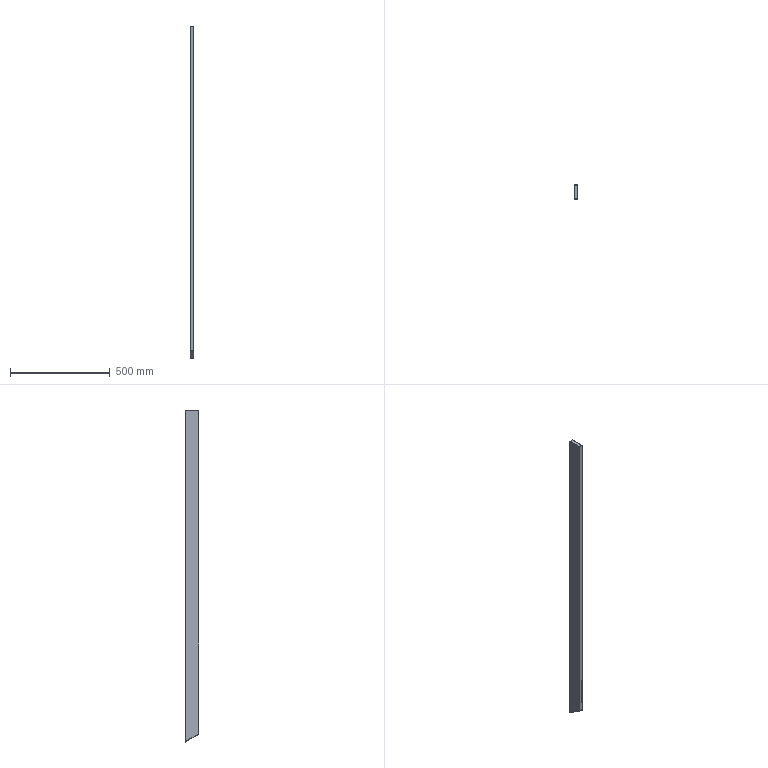Part | SolidWorks | features ICE 8, EdgeFlange 2, FlatPattern 1, LPattern 1, SMBaseFlange 1, SheetMetal 1 | 1 solid | 79 faces | box 20 x 70 x 1667 mm | volume 353631 mm3 | plane 46 | cylinder 28 | spline 5 | commonest cylinder face diameters 6.4 x16 1 x6 4 x6